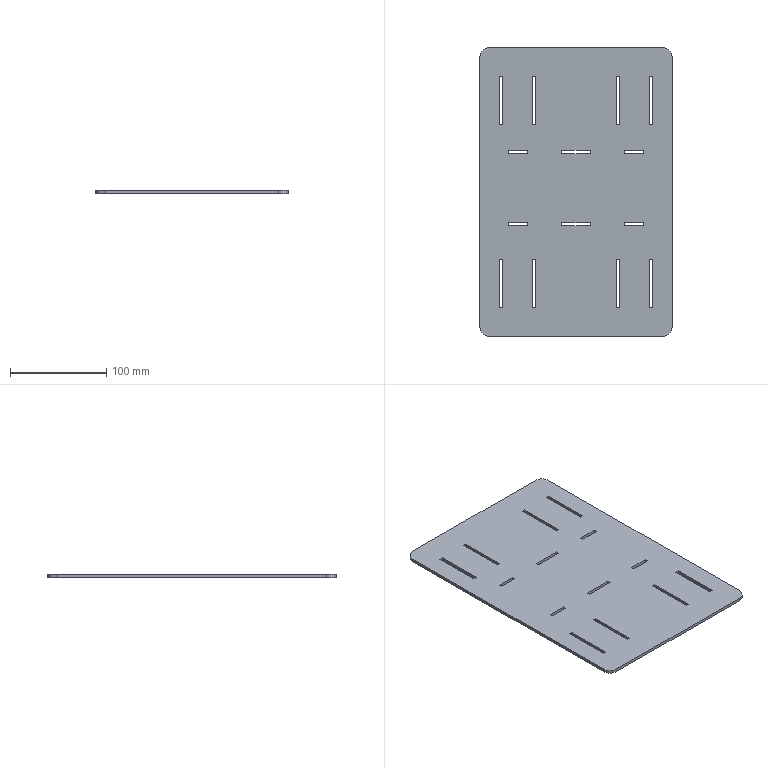Part | SolidWorks | features FlatPattern 1, SMBaseFlange 1, SheetMetal 1 | 1 solid | 66 faces | box 200 x 300 x 3.2 mm | volume 186196 mm3 | plane 62 | cylinder 4 | commonest cylinder face diameters 20 x4